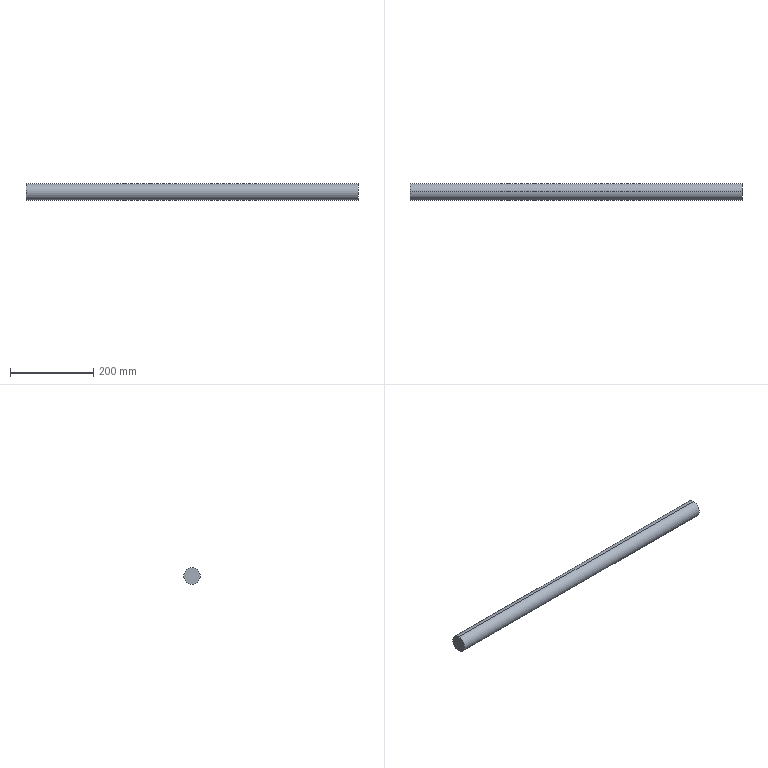Part | SolidWorks | features Extrusion 1 | 1 solid | 4 faces | box 800 x 40 x 40 mm | volume 1005310 mm3 | cylinder 2 | plane 2 | commonest cylinder face diameters 40 x2
STEP:
#1=CARTESIAN_POINT('',(800.,0.,-20.));
#2=VERTEX_POINT('',#1);
#3=CARTESIAN_POINT('',(800.,0.,20.));
#4=VERTEX_POINT('',#3);
#5=CARTESIAN_POINT('',(800.,0.,0.));
#6=DIRECTION('',(1.,0.,0.));
#7=DIRECTION('',(0.,0.,-1.));
#8=AXIS2_PLACEMENT_3D('',#5,#6,#7);
#9=CIRCLE('',#8,20.);
#10=EDGE_CURVE('',#2,#4,#9,.T.);
#11=ORIENTED_EDGE('',*,*,#10,.F.);
#12=CARTESIAN_POINT('',(0.,0.,-20.));
#13=VERTEX_POINT('',#12);
#14=CARTESIAN_POINT('',(800.,0.,-20.));
#15=DIRECTION('',(-1.,0.,0.));
#16=VECTOR('',#15,1000.);
#17=LINE('',#14,#16);
#18=EDGE_CURVE('',#2,#13,#17,.T.);
#19=ORIENTED_EDGE('',*,*,#18,.T.);
#20=CARTESIAN_POINT('',(0.,0.,20.));
#21=VERTEX_POINT('',#20);
#22=CARTESIAN_POINT('',(0.,0.,0.));
#23=DIRECTION('',(1.,0.,0.));
#24=DIRECTION('',(0.,0.,-1.));
#25=AXIS2_PLACEMENT_3D('',#22,#23,#24);
#26=CIRCLE('',#25,20.);
#27=EDGE_CURVE('',#13,#21,#26,.T.);
#28=ORIENTED_EDGE('',*,*,#27,.T.);
#29=CARTESIAN_POINT('',(800.,0.,20.));
#30=DIRECTION('',(-1.,0.,0.));
#31=VECTOR('',#30,1000.);
#32=LINE('',#29,#31);
#33=EDGE_CURVE('',#4,#21,#32,.T.);
#34=ORIENTED_EDGE('',*,*,#33,.F.);
#35=EDGE_LOOP('',(#11,#19,#28,#34));
#36=FACE_OUTER_BOUND('',#35,.T.);
#37=CARTESIAN_POINT('',(800.,0.,0.));
#38=DIRECTION('',(-1.,0.,0.));
#39=DIRECTION('',(0.,0.,1.));
#40=AXIS2_PLACEMENT_3D('',#37,#38,#39);
#41=CYLINDRICAL_SURFACE('',#40,20.);
#42=ADVANCED_FACE('',(#36),#41,.T.);
#43=ORIENTED_EDGE('',*,*,#18,.F.);
#44=CARTESIAN_POINT('',(800.,0.,0.));
#45=DIRECTION('',(1.,0.,0.));
#46=DIRECTION('',(0.,0.,-1.));
#47=AXIS2_PLACEMENT_3D('',#44,#45,#46);
#48=CIRCLE('',#47,20.);
#49=EDGE_CURVE('',#4,#2,#48,.T.);
#50=ORIENTED_EDGE('',*,*,#49,.F.);
#51=ORIENTED_EDGE('',*,*,#33,.T.);
#52=CARTESIAN_POINT('',(0.,0.,0.));
#53=DIRECTION('',(1.,0.,0.));
#54=DIRECTION('',(0.,0.,-1.));
#55=AXIS2_PLACEMENT_3D('',#52,#53,#54);
#56=CIRCLE('',#55,20.);
#57=EDGE_CURVE('',#21,#13,#56,.T.);
#58=ORIENTED_EDGE('',*,*,#57,.T.);
#59=EDGE_LOOP('',(#43,#50,#51,#58));
#60=FACE_OUTER_BOUND('',#59,.T.);
#61=CARTESIAN_POINT('',(800.,0.,0.));
#62=DIRECTION('',(-1.,0.,0.));
#63=DIRECTION('',(0.,0.,1.));
#64=AXIS2_PLACEMENT_3D('',#61,#62,#63);
#65=CYLINDRICAL_SURFACE('',#64,20.);
#66=ADVANCED_FACE('',(#60),#65,.T.);
#67=ORIENTED_EDGE('',*,*,#49,.T.);
#68=ORIENTED_EDGE('',*,*,#10,.T.);
#69=EDGE_LOOP('',(#67,#68));
#70=FACE_OUTER_BOUND('',#69,.T.);
#71=CARTESIAN_POINT('',(800.,0.,0.));
#72=DIRECTION('',(1.,0.,0.));
#73=DIRECTION('',(0.,0.,-1.));
#74=AXIS2_PLACEMENT_3D('',#71,#72,#73);
#75=PLANE('',#74);
#76=ADVANCED_FACE('',(#70),#75,.T.);
#77=ORIENTED_EDGE('',*,*,#57,.F.);
#78=ORIENTED_EDGE('',*,*,#27,.F.);
#79=EDGE_LOOP('',(#77,#78));
#80=FACE_OUTER_BOUND('',#79,.T.);
#81=CARTESIAN_POINT('',(0.,0.,0.));
#82=DIRECTION('',(1.,0.,0.));
#83=DIRECTION('',(0.,0.,-1.));
#84=AXIS2_PLACEMENT_3D('',#81,#82,#83);
#85=PLANE('',#84);
#86=ADVANCED_FACE('',(#80),#85,.F.);
#87=CLOSED_SHELL('',(#42,#66,#76,#86));
#88=MANIFOLD_SOLID_BREP('',#87);
#89=CARTESIAN_POINT('',(0.,0.,0.));
#90=DIRECTION('',(0.,0.,1.));
#91=DIRECTION('',(1.,0.,0.));
#92=AXIS2_PLACEMENT_3D('',#89,#90,#91);
#93=(LENGTH_UNIT()NAMED_UNIT(*)SI_UNIT(.MILLI.,.METRE.));
#94=UNCERTAINTY_MEASURE_WITH_UNIT(LENGTH_MEASURE(0.00001),#93,'','');
#95=(NAMED_UNIT(*)PLANE_ANGLE_UNIT()SI_UNIT($,.RADIAN.));
#96=(NAMED_UNIT(*)SI_UNIT($,.STERADIAN.)SOLID_ANGLE_UNIT());
#97=(GEOMETRIC_REPRESENTATION_CONTEXT(3)GLOBAL_UNCERTAINTY_ASSIGNED_CONTEXT((#94))GLOBAL_UNIT_ASSIGNED_CONTEXT((#93,#95,#96))REPRESENTATION_CONTEXT('',''));
#98=ADVANCED_BREP_SHAPE_REPRESENTATION('',(#88,#92),#97);